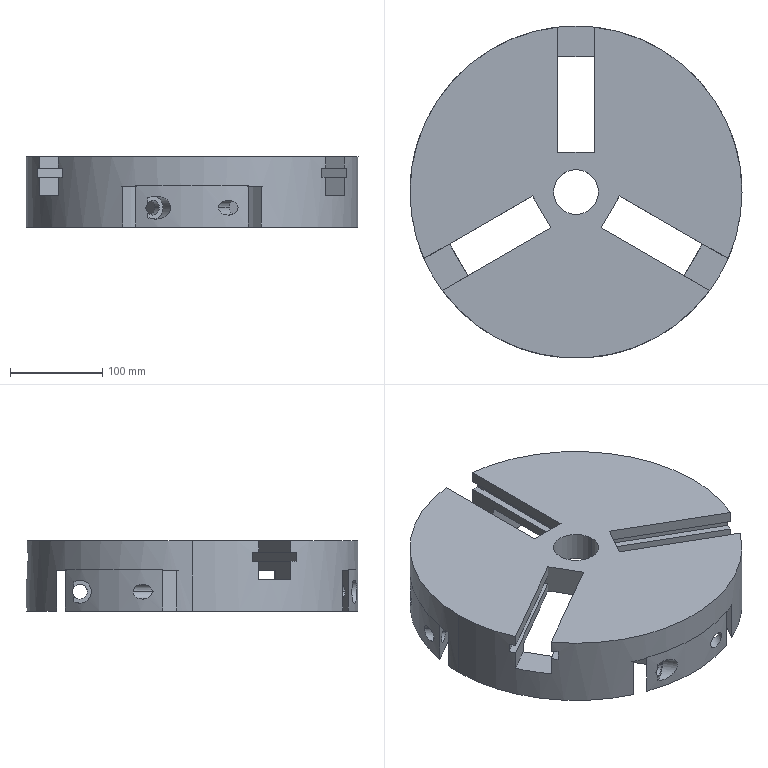Part | SolidWorks | features ICE 10, CirPattern 5, Cut 1, Extrusion 1 | 3 solids | 100 faces | box 360 x 360 x 76 mm | volume 3930105 mm3 | plane 74 | cylinder 26 | commonest cylinder face diameters 16 x12 205 x5 360 x4 25 x3 48.592 x2